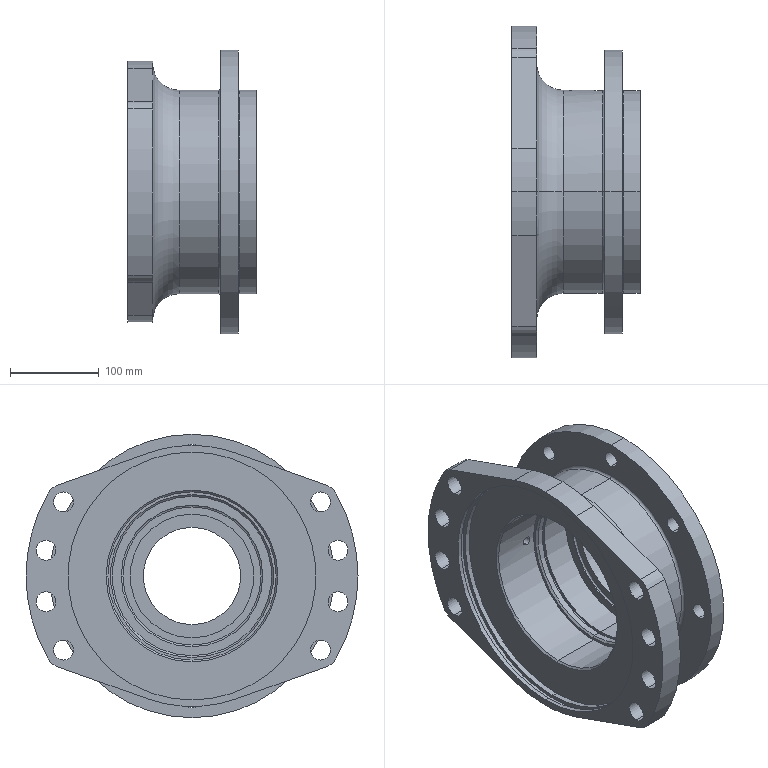Part | SolidWorks | features ICE 2, 3DProfileFeature 1, CirPattern 1, HoleWzd 1, Revolution 1 | 1 solid | 102 faces | box 145 x 375 x 320 mm | volume 3842177 mm3 | cylinder 71 | plane 19 | torus 8 | cone 4 | commonest cylinder face diameters 18 x16 22.5 x16 40 x4 180 x4 230 x4 280 x4